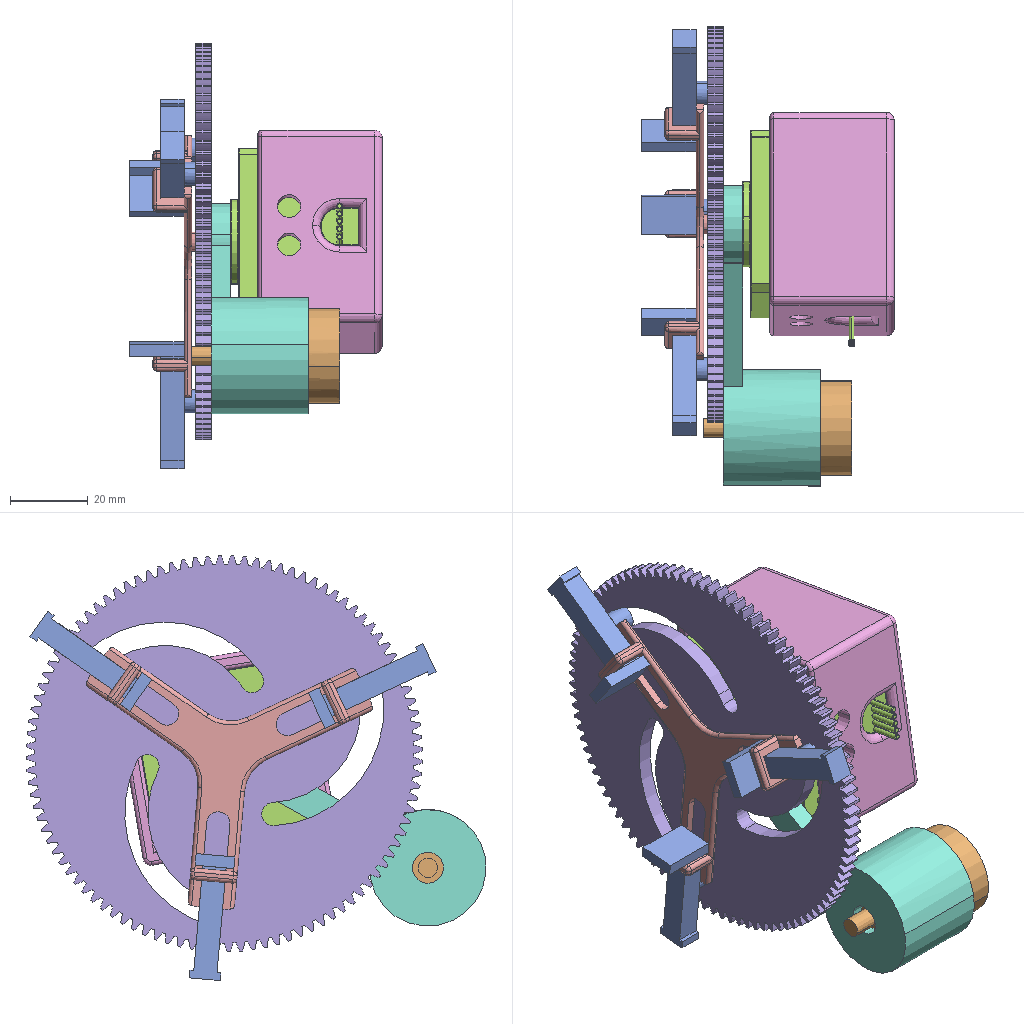Assembly | SolidWorks | 7 different items | 9 placed | box 65 x 118 x 109 mm
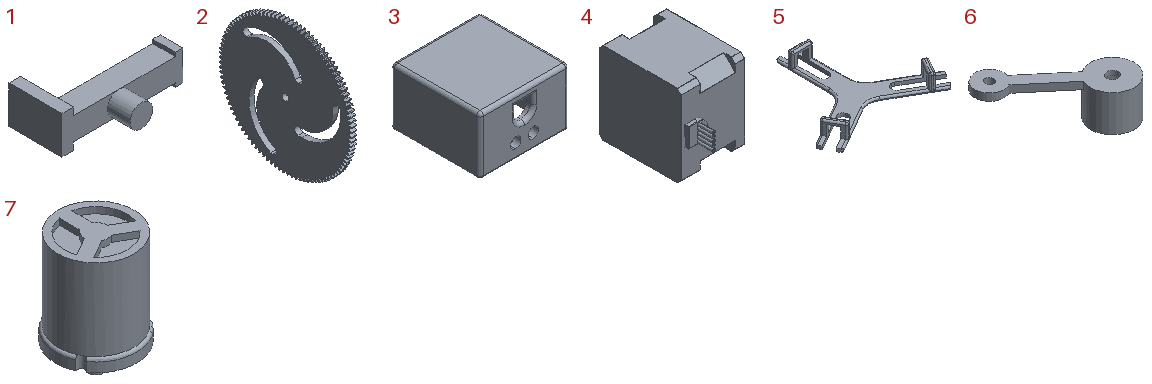Parts list (item | quantity | size | volume | features):
1 | x3 | 32 x 20 x 10 mm | 1658 mm3 | features ICE 5, Extrusion 1
2 | x1 | 4 x 101.968 x 101.968 mm | 27433 mm3 | features BaseBody 1
3 | x1 | 50.3 x 50.3 x 32 mm | 29890 mm3 | features Fillet 3, Cut 1, Extrusion 1, HoleWzd 1, ICE 1
4 | x1 | 37 x 52.3 x 42.3 mm | 58361 mm3 | features Revolution 6, ICE 5, HoleWzd 2, Extrusion 1, Fillet 1
5 | x1 | 73.993 x 64.557 x 18 mm | 2470 mm3 | features ICE 4, Fillet 3, CirPattern 1, Extrusion 1
6 | x1 | 70.91 x 63.63 x 25 mm | 8702 mm3 | features ICE 3, Extrusion 1
7 | x1 | 26 x 25.935 x 38 mm | 13857 mm3 | features ICE 6, Fillet 2, Extrusion 1
Mates (type | each side: item.copy, entity, surface, feature):
Parallel | 5.1 face plane CirPattern1 | 1.1 face plane Boss-Extrude1
Coincident | 5.1 face plane CirPattern1 | 1.1 face plane Boss-Extrude1 | 2 times
Coincident | 5.1 face plane Cut-Extrude1 | 1.2 face plane Boss-Extrude1 | 2 times
Coincident | 5.1 face plane CirPattern1 | 1.3 face plane Boss-Extrude1 | 2 times
Concentric | 5.1 face cylinder Boss-Extrude3 | 4.1 edge
Coincident | 5.1 face plane Boss-Extrude3 | 4.1 face plane Cut-Extrude1
InPlace | 4.1 face plane Boss-Extrude3 | 3.1 plane
Concentric | 5.1 face cylinder Boss-Extrude3 | 6.1 face cylinder Boss-Extrude1
Coincident | 4.1 face plane Boss-Extrude5 | 6.1 face plane Boss-Extrude1
Lock | 5.1 select_type:0 | 6.1 select_type:0
Concentric | 7.1 face cylinder Boss-Extrude2 | assembly face | 2 times
Concentric | 6.1 face cylinder Cut-Extrude1 | 7.1 face cylinder Boss-Extrude1
Coincident | 6.1 face plane Cut-Extrude1 | 7.1 face plane Boss-Extrude1
Concentric | 5.1 face cylinder Boss-Extrude3 | 2.1 face cylinder Input1
Coincident | 6.1 face plane Boss-Extrude1 | 2.1 face plane Input1
Tangent | 1.3 face cylinder Boss-Extrude2 | 2.1 face cylinder Input1
Tangent | 1.1 face cylinder Boss-Extrude2 | 2.1 face cylinder Input1
Tangent | 1.2 face cylinder Boss-Extrude2 | 2.1 face cylinder Input1
Coincident | 6.1 face plane Boss-Extrude1 | assembly face
GearDim | assembly face | 2.1 face cylinder Input1
Concentric | 1.3 face cylinder Boss-Extrude2 | 2.1 face cylinder Input1